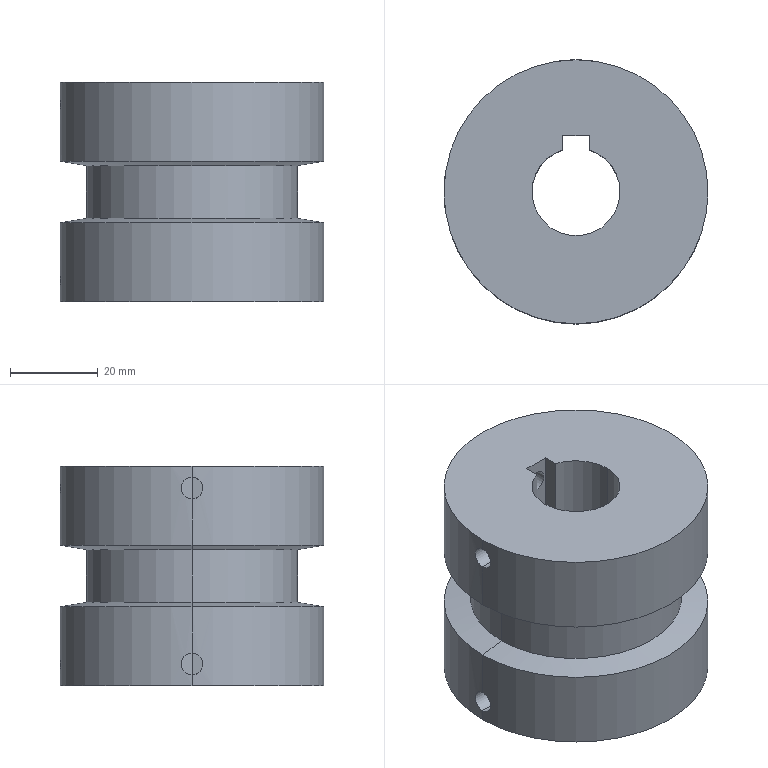Part | STEP file | ENE11-D60-N20-L50-X14-Y12-Z5 flat belt pulley Yihda 171 | 1 solid | 26 faces | box 60 x 60 x 50 mm | volume 110095 mm3 | cylinder 17 | plane 5 | cone 4 | commonest cylinder face diameters 4.917 x8 60 x4 20 x3 48 x2
STEP:
#1=CARTESIAN_POINT('',(-10.,0.,-50.));
#2=VERTEX_POINT('',#1);
#3=CARTESIAN_POINT('',(-3.,9.539,-50.));
#4=VERTEX_POINT('',#3);
#5=CARTESIAN_POINT('',(0.,0.,-50.));
#6=DIRECTION('',(0.,0.,-1.));
#7=DIRECTION('',(-1.,0.,0.));
#8=AXIS2_PLACEMENT_3D('',#5,#6,#7);
#9=CIRCLE('',#8,10.);
#10=EDGE_CURVE('',#2,#4,#9,.T.);
#11=ORIENTED_EDGE('',*,*,#10,.T.);
#12=CARTESIAN_POINT('',(-3.,9.539,0.));
#13=VERTEX_POINT('',#12);
#14=CARTESIAN_POINT('',(-3.,9.539,-50.));
#15=DIRECTION('',(0.,0.,1.));
#16=VECTOR('',#15,1000.);
#17=LINE('',#14,#16);
#18=EDGE_CURVE('',#4,#13,#17,.T.);
#19=ORIENTED_EDGE('',*,*,#18,.T.);
#20=CARTESIAN_POINT('',(-10.,0.,0.));
#21=VERTEX_POINT('',#20);
#22=CARTESIAN_POINT('',(0.,0.,0.));
#23=DIRECTION('',(0.,0.,-1.));
#24=DIRECTION('',(-1.,0.,0.));
#25=AXIS2_PLACEMENT_3D('',#22,#23,#24);
#26=CIRCLE('',#25,10.);
#27=EDGE_CURVE('',#21,#13,#26,.T.);
#28=ORIENTED_EDGE('',*,*,#27,.F.);
#29=CARTESIAN_POINT('',(-10.,0.,-2.542));
#30=VERTEX_POINT('',#29);
#31=CARTESIAN_POINT('',(-10.,0.,-2.542));
#32=DIRECTION('',(0.,0.,1.));
#33=VECTOR('',#32,1000.);
#34=LINE('',#31,#33);
#35=EDGE_CURVE('',#30,#21,#34,.T.);
#36=ORIENTED_EDGE('',*,*,#35,.F.);
#37=CARTESIAN_POINT('',(-10.,0.,-7.458));
#38=VERTEX_POINT('',#37);
#39=CARTESIAN_POINT('',(-10.,0.,-2.542));
#40=CARTESIAN_POINT('',(-10.,0.1631,-2.542));
#41=CARTESIAN_POINT('',(-9.996,0.3233,-2.558));
#42=CARTESIAN_POINT('',(-9.981,0.6386,-2.62));
#43=CARTESIAN_POINT('',(-9.969,0.795,-2.668));
#44=CARTESIAN_POINT('',(-9.941,1.092,-2.792));
#45=CARTESIAN_POINT('',(-9.925,1.233,-2.867));
#46=CARTESIAN_POINT('',(-9.888,1.5,-3.046));
#47=CARTESIAN_POINT('',(-9.868,1.626,-3.149));
#48=CARTESIAN_POINT('',(-9.808,1.965,-3.488));
#49=CARTESIAN_POINT('',(-9.768,2.148,-3.761));
#50=CARTESIAN_POINT('',(-9.725,2.332,-4.205));
#51=CARTESIAN_POINT('',(-9.713,2.379,-4.36));
#52=CARTESIAN_POINT('',(-9.697,2.443,-4.678));
#53=CARTESIAN_POINT('',(-9.693,2.458,-4.838));
#54=CARTESIAN_POINT('',(-9.693,2.459,-5.16));
#55=CARTESIAN_POINT('',(-9.697,2.442,-5.324));
#56=CARTESIAN_POINT('',(-9.713,2.379,-5.64));
#57=CARTESIAN_POINT('',(-9.724,2.333,-5.793));
#58=CARTESIAN_POINT('',(-9.768,2.147,-6.24));
#59=CARTESIAN_POINT('',(-9.808,1.966,-6.511));
#60=CARTESIAN_POINT('',(-9.868,1.624,-6.853));
#61=CARTESIAN_POINT('',(-9.888,1.501,-6.954));
#62=CARTESIAN_POINT('',(-9.924,1.235,-7.132));
#63=CARTESIAN_POINT('',(-9.941,1.091,-7.209));
#64=CARTESIAN_POINT('',(-9.97,0.7939,-7.332));
#65=CARTESIAN_POINT('',(-9.981,0.6406,-7.379));
#66=CARTESIAN_POINT('',(-9.996,0.3241,-7.442));
#67=CARTESIAN_POINT('',(-10.,0.1608,-7.459));
#68=CARTESIAN_POINT('',(-10.,0.,-7.458));
#69=B_SPLINE_CURVE_WITH_KNOTS('',3,(#39,#40,#41,#42,#43,#44,#45,#46,#47,#48,#49,#50,#51,#52,#53,#54,#55,#56,#57,#58,#59,#60,#61,#62,#63,#64,#65,#66,#67,#68),.UNSPECIFIED.,.F.,.F.,(4,2,2,2,2,2,2,2,2,2,2,2,2,2,4),(0.,0.0004823,0.0009645,0.001447,0.001929,0.002894,0.003376,0.003858,0.00434,0.004823,0.005787,0.006269,0.006752,0.007234,0.007716),.UNSPECIFIED.);
#70=EDGE_CURVE('',#30,#38,#69,.T.);
#71=ORIENTED_EDGE('',*,*,#70,.T.);
#72=CARTESIAN_POINT('',(-10.,-0.000000171,-7.458));
#73=VERTEX_POINT('',#72);
#74=CARTESIAN_POINT('',(-10.,0.,-7.458));
#75=DIRECTION('',(0.00006947,-1.,0.000000036));
#76=VECTOR('',#75,1000.);
#77=LINE('',#74,#76);
#78=EDGE_CURVE('',#38,#73,#77,.T.);
#79=ORIENTED_EDGE('',*,*,#78,.T.);
#80=CARTESIAN_POINT('',(-10.,0.,-42.542));
#81=VERTEX_POINT('',#80);
#82=CARTESIAN_POINT('',(-10.,0.,-42.542));
#83=DIRECTION('',(0.,0.,1.));
#84=VECTOR('',#83,1000.);
#85=LINE('',#82,#84);
#86=EDGE_CURVE('',#81,#73,#85,.T.);
#87=ORIENTED_EDGE('',*,*,#86,.F.);
#88=CARTESIAN_POINT('',(-10.,0.,-47.458));
#89=VERTEX_POINT('',#88);
#90=CARTESIAN_POINT('',(-10.,0.,-42.542));
#91=CARTESIAN_POINT('',(-10.,0.1631,-42.542));
#92=CARTESIAN_POINT('',(-9.996,0.3233,-42.558));
#93=CARTESIAN_POINT('',(-9.981,0.6386,-42.62));
#94=CARTESIAN_POINT('',(-9.969,0.795,-42.668));
#95=CARTESIAN_POINT('',(-9.941,1.092,-42.792));
#96=CARTESIAN_POINT('',(-9.925,1.233,-42.867));
#97=CARTESIAN_POINT('',(-9.888,1.5,-43.046));
#98=CARTESIAN_POINT('',(-9.868,1.626,-43.149));
#99=CARTESIAN_POINT('',(-9.808,1.965,-43.488));
#100=CARTESIAN_POINT('',(-9.768,2.148,-43.761));
#101=CARTESIAN_POINT('',(-9.725,2.332,-44.205));
#102=CARTESIAN_POINT('',(-9.713,2.379,-44.36));
#103=CARTESIAN_POINT('',(-9.697,2.443,-44.678));
#104=CARTESIAN_POINT('',(-9.693,2.458,-44.838));
#105=CARTESIAN_POINT('',(-9.693,2.459,-45.16));
#106=CARTESIAN_POINT('',(-9.697,2.442,-45.324));
#107=CARTESIAN_POINT('',(-9.713,2.379,-45.64));
#108=CARTESIAN_POINT('',(-9.724,2.333,-45.793));
#109=CARTESIAN_POINT('',(-9.768,2.147,-46.24));
#110=CARTESIAN_POINT('',(-9.808,1.966,-46.511));
#111=CARTESIAN_POINT('',(-9.868,1.624,-46.853));
#112=CARTESIAN_POINT('',(-9.888,1.501,-46.954));
#113=CARTESIAN_POINT('',(-9.924,1.235,-47.132));
#114=CARTESIAN_POINT('',(-9.941,1.091,-47.209));
#115=CARTESIAN_POINT('',(-9.97,0.7939,-47.332));
#116=CARTESIAN_POINT('',(-9.981,0.6406,-47.379));
#117=CARTESIAN_POINT('',(-9.996,0.324,-47.442));
#118=CARTESIAN_POINT('',(-10.,0.1611,-47.459));
#119=CARTESIAN_POINT('',(-10.,0.,-47.458));
#120=B_SPLINE_CURVE_WITH_KNOTS('',3,(#90,#91,#92,#93,#94,#95,#96,#97,#98,#99,#100,#101,#102,#103,#104,#105,#106,#107,#108,#109,#110,#111,#112,#113,#114,#115,#116,#117,#118,#119),.UNSPECIFIED.,.F.,.F.,(4,2,2,2,2,2,2,2,2,2,2,2,2,2,4),(0.,0.0004823,0.0009645,0.001447,0.001929,0.002894,0.003376,0.003858,0.00434,0.004823,0.005787,0.006269,0.006752,0.007234,0.007716),.UNSPECIFIED.);
#121=EDGE_CURVE('',#81,#89,#120,.T.);
#122=ORIENTED_EDGE('',*,*,#121,.T.);
#123=CARTESIAN_POINT('',(-10.,0.,-50.));
#124=DIRECTION('',(0.,0.,1.));
#125=VECTOR('',#124,1000.);
#126=LINE('',#123,#125);
#127=EDGE_CURVE('',#2,#89,#126,.T.);
#128=ORIENTED_EDGE('',*,*,#127,.F.);
#129=EDGE_LOOP('',(#11,#19,#28,#36,#71,#79,#87,#122,#128));
#130=FACE_OUTER_BOUND('',#129,.T.);
#131=CARTESIAN_POINT('',(0.,0.,-50.));
#132=DIRECTION('',(0.,0.,1.));
#133=DIRECTION('',(0.,-1.,0.));
#134=AXIS2_PLACEMENT_3D('',#131,#132,#133);
#135=CYLINDRICAL_SURFACE('',#134,10.);
#136=ADVANCED_FACE('',(#130),#135,.F.);
#137=ORIENTED_EDGE('',*,*,#70,.F.);
#138=CARTESIAN_POINT('',(-30.,0.,-2.541));
#139=VERTEX_POINT('',#138);
#140=CARTESIAN_POINT('',(-10.,0.,-2.542));
#141=DIRECTION('',(-1.,0.,0.));
#142=VECTOR('',#141,1000.);
#143=LINE('',#140,#142);
#144=EDGE_CURVE('',#30,#139,#143,.T.);
#145=ORIENTED_EDGE('',*,*,#144,.T.);
#146=CARTESIAN_POINT('',(-30.,0.,-7.458));
#147=VERTEX_POINT('',#146);
#148=CARTESIAN_POINT('',(-30.,0.,-7.458));
#149=CARTESIAN_POINT('',(-30.,0.1625,-7.458));
#150=CARTESIAN_POINT('',(-29.999,0.3222,-7.443));
#151=CARTESIAN_POINT('',(-29.994,0.6368,-7.38));
#152=CARTESIAN_POINT('',(-29.99,0.7928,-7.333));
#153=CARTESIAN_POINT('',(-29.981,1.091,-7.209));
#154=CARTESIAN_POINT('',(-29.975,1.232,-7.134));
#155=CARTESIAN_POINT('',(-29.963,1.499,-6.955));
#156=CARTESIAN_POINT('',(-29.956,1.625,-6.852));
#157=CARTESIAN_POINT('',(-29.943,1.852,-6.625));
#158=CARTESIAN_POINT('',(-29.936,1.954,-6.501));
#159=CARTESIAN_POINT('',(-29.924,2.133,-6.232));
#160=CARTESIAN_POINT('',(-29.919,2.21,-6.089));
#161=CARTESIAN_POINT('',(-29.909,2.333,-5.793));
#162=CARTESIAN_POINT('',(-29.905,2.38,-5.638));
#163=CARTESIAN_POINT('',(-29.9,2.443,-5.321));
#164=CARTESIAN_POINT('',(-29.899,2.458,-5.161));
#165=CARTESIAN_POINT('',(-29.899,2.459,-4.84));
#166=CARTESIAN_POINT('',(-29.9,2.443,-4.678));
#167=CARTESIAN_POINT('',(-29.905,2.38,-4.362));
#168=CARTESIAN_POINT('',(-29.909,2.333,-4.209));
#169=CARTESIAN_POINT('',(-29.919,2.21,-3.911));
#170=CARTESIAN_POINT('',(-29.924,2.133,-3.767));
#171=CARTESIAN_POINT('',(-29.936,1.955,-3.501));
#172=CARTESIAN_POINT('',(-29.943,1.853,-3.377));
#173=CARTESIAN_POINT('',(-29.956,1.624,-3.147));
#174=CARTESIAN_POINT('',(-29.963,1.5,-3.045));
#175=CARTESIAN_POINT('',(-29.975,1.233,-2.867));
#176=CARTESIAN_POINT('',(-29.981,1.09,-2.79));
#177=CARTESIAN_POINT('',(-29.99,0.792,-2.667));
#178=CARTESIAN_POINT('',(-29.994,0.6387,-2.62));
#179=CARTESIAN_POINT('',(-29.999,0.3234,-2.558));
#180=CARTESIAN_POINT('',(-30.,0.1606,-2.542));
#181=CARTESIAN_POINT('',(-30.,0.,-2.541));
#182=B_SPLINE_CURVE_WITH_KNOTS('',3,(#148,#149,#150,#151,#152,#153,#154,#155,#156,#157,#158,#159,#160,#161,#162,#163,#164,#165,#166,#167,#168,#169,#170,#171,#172,#173,#174,#175,#176,#177,#178,#179,#180,#181),.UNSPECIFIED.,.F.,.F.,(4,2,2,2,2,2,2,2,2,2,2,2,2,2,2,2,4),(0.,0.0004806,0.0009612,0.001442,0.001922,0.002403,0.002884,0.003364,0.003845,0.004325,0.004806,0.005287,0.005767,0.006248,0.006728,0.007209,0.00769),.UNSPECIFIED.);
#183=EDGE_CURVE('',#147,#139,#182,.T.);
#184=ORIENTED_EDGE('',*,*,#183,.F.);
#185=CARTESIAN_POINT('',(-10.,0.,-7.458));
#186=DIRECTION('',(-1.,0.,0.));
#187=VECTOR('',#186,1000.);
#188=LINE('',#185,#187);
#189=EDGE_CURVE('',#38,#147,#188,.T.);
#190=ORIENTED_EDGE('',*,*,#189,.F.);
#191=EDGE_LOOP('',(#137,#145,#184,#190));
#192=FACE_OUTER_BOUND('',#191,.T.);
#193=CARTESIAN_POINT('',(0.,0.,-5.));
#194=DIRECTION('',(-1.,0.,0.));
#195=DIRECTION('',(0.,-1.,0.));
#196=AXIS2_PLACEMENT_3D('',#193,#194,#195);
#197=CYLINDRICAL_SURFACE('',#196,2.459);
#198=ADVANCED_FACE('',(#192),#197,.F.);
#199=CARTESIAN_POINT('',(-30.,0.,-2.541));
#200=CARTESIAN_POINT('',(-30.,-0.1606,-2.541));
#201=CARTESIAN_POINT('',(-29.999,-0.3201,-2.557));
#202=CARTESIAN_POINT('',(-29.994,-0.6369,-2.62));
#203=CARTESIAN_POINT('',(-29.99,-0.7923,-2.667));
#204=CARTESIAN_POINT('',(-29.976,-1.236,-2.851));
#205=CARTESIAN_POINT('',(-29.963,-1.51,-3.034));
#206=CARTESIAN_POINT('',(-29.943,-1.851,-3.374));
#207=CARTESIAN_POINT('',(-29.936,-1.954,-3.5));
#208=CARTESIAN_POINT('',(-29.924,-2.133,-3.767));
#209=CARTESIAN_POINT('',(-29.919,-2.209,-3.908));
#210=CARTESIAN_POINT('',(-29.909,-2.332,-4.206));
#211=CARTESIAN_POINT('',(-29.905,-2.38,-4.362));
#212=CARTESIAN_POINT('',(-29.9,-2.442,-4.676));
#213=CARTESIAN_POINT('',(-29.899,-2.458,-4.836));
#214=CARTESIAN_POINT('',(-29.899,-2.459,-5.16));
#215=CARTESIAN_POINT('',(-29.9,-2.443,-5.32));
#216=CARTESIAN_POINT('',(-29.905,-2.38,-5.635));
#217=CARTESIAN_POINT('',(-29.909,-2.333,-5.791));
#218=CARTESIAN_POINT('',(-29.919,-2.21,-6.089));
#219=CARTESIAN_POINT('',(-29.924,-2.135,-6.23));
#220=CARTESIAN_POINT('',(-29.936,-1.957,-6.497));
#221=CARTESIAN_POINT('',(-29.943,-1.853,-6.624));
#222=CARTESIAN_POINT('',(-29.956,-1.626,-6.851));
#223=CARTESIAN_POINT('',(-29.963,-1.503,-6.953));
#224=CARTESIAN_POINT('',(-29.975,-1.234,-7.132));
#225=CARTESIAN_POINT('',(-29.981,-1.091,-7.209));
#226=CARTESIAN_POINT('',(-29.994,-0.6476,-7.393));
#227=CARTESIAN_POINT('',(-30.,-0.3249,-7.458));
#228=CARTESIAN_POINT('',(-30.,0.,-7.458));
#229=B_SPLINE_CURVE_WITH_KNOTS('',3,(#199,#200,#201,#202,#203,#204,#205,#206,#207,#208,#209,#210,#211,#212,#213,#214,#215,#216,#217,#218,#219,#220,#221,#222,#223,#224,#225,#226,#227,#228),.UNSPECIFIED.,.F.,.F.,(4,2,2,2,2,2,2,2,2,2,2,2,2,2,4),(0.00769,0.00817,0.008651,0.009612,0.01009,0.01057,0.01105,0.01153,0.01201,0.01249,0.01297,0.01346,0.01394,0.01442,0.01538),.UNSPECIFIED.);
#230=EDGE_CURVE('',#139,#147,#229,.T.);
#231=ORIENTED_EDGE('',*,*,#230,.F.);
#232=ORIENTED_EDGE('',*,*,#144,.F.);
#233=CARTESIAN_POINT('',(-10.,-0.000000171,-7.458));
#234=CARTESIAN_POINT('',(-10.,-0.3216,-7.458));
#235=CARTESIAN_POINT('',(-9.984,-0.6459,-7.394));
#236=CARTESIAN_POINT('',(-9.941,-1.091,-7.209));
#237=CARTESIAN_POINT('',(-9.924,-1.234,-7.132));
#238=CARTESIAN_POINT('',(-9.888,-1.501,-6.954));
#239=CARTESIAN_POINT('',(-9.868,-1.624,-6.852));
#240=CARTESIAN_POINT('',(-9.828,-1.851,-6.626));
#241=CARTESIAN_POINT('',(-9.808,-1.954,-6.5));
#242=CARTESIAN_POINT('',(-9.77,-2.132,-6.234));
#243=CARTESIAN_POINT('',(-9.753,-2.208,-6.093));
#244=CARTESIAN_POINT('',(-9.71,-2.394,-5.645));
#245=CARTESIAN_POINT('',(-9.693,-2.458,-5.325));
#246=CARTESIAN_POINT('',(-9.693,-2.459,-4.839));
#247=CARTESIAN_POINT('',(-9.697,-2.443,-4.679));
#248=CARTESIAN_POINT('',(-9.713,-2.38,-4.363));
#249=CARTESIAN_POINT('',(-9.724,-2.332,-4.206));
#250=CARTESIAN_POINT('',(-9.753,-2.209,-3.909));
#251=CARTESIAN_POINT('',(-9.77,-2.134,-3.768));
#252=CARTESIAN_POINT('',(-9.807,-1.955,-3.5));
#253=CARTESIAN_POINT('',(-9.828,-1.852,-3.376));
#254=CARTESIAN_POINT('',(-9.887,-1.514,-3.037));
#255=CARTESIAN_POINT('',(-9.927,-1.241,-2.854));
#256=CARTESIAN_POINT('',(-9.969,-0.7971,-2.669));
#257=CARTESIAN_POINT('',(-9.981,-0.6407,-2.621));
#258=CARTESIAN_POINT('',(-9.996,-0.3238,-2.558));
#259=CARTESIAN_POINT('',(-10.,-0.1631,-2.542));
#260=CARTESIAN_POINT('',(-10.,0.,-2.542));
#261=B_SPLINE_CURVE_WITH_KNOTS('',3,(#233,#234,#235,#236,#237,#238,#239,#240,#241,#242,#243,#244,#245,#246,#247,#248,#249,#250,#251,#252,#253,#254,#255,#256,#257,#258,#259,#260),.UNSPECIFIED.,.F.,.F.,(4,2,2,2,2,2,2,2,2,2,2,2,2,4),(0.007716,0.00868,0.009162,0.009645,0.01013,0.01061,0.01157,0.01206,0.01254,0.01302,0.0135,0.01447,0.01495,0.01543),.UNSPECIFIED.);
#262=EDGE_CURVE('',#73,#30,#261,.T.);
#263=ORIENTED_EDGE('',*,*,#262,.F.);
#264=ORIENTED_EDGE('',*,*,#78,.F.);
#265=ORIENTED_EDGE('',*,*,#189,.T.);
#266=EDGE_LOOP('',(#231,#232,#263,#264,#265));
#267=FACE_OUTER_BOUND('',#266,.T.);
#268=CARTESIAN_POINT('',(0.,0.,-5.));
#269=DIRECTION('',(-1.,0.,0.));
#270=DIRECTION('',(0.,1.,0.));
#271=AXIS2_PLACEMENT_3D('',#268,#269,#270);
#272=CYLINDRICAL_SURFACE('',#271,2.459);
#273=ADVANCED_FACE('',(#267),#272,.F.);
#274=CARTESIAN_POINT('',(3.,9.539,0.));
#275=VERTEX_POINT('',#274);
#276=CARTESIAN_POINT('',(10.,0.,0.));
#277=VERTEX_POINT('',#276);
#278=CARTESIAN_POINT('',(0.,0.,0.));
#279=DIRECTION('',(0.,0.,-1.));
#280=DIRECTION('',(-1.,0.,0.));
#281=AXIS2_PLACEMENT_3D('',#278,#279,#280);
#282=CIRCLE('',#281,10.);
#283=EDGE_CURVE('',#275,#277,#282,.T.);
#284=ORIENTED_EDGE('',*,*,#283,.F.);
#285=CARTESIAN_POINT('',(3.,9.539,-50.));
#286=VERTEX_POINT('',#285);
#287=CARTESIAN_POINT('',(3.,9.539,-50.));
#288=DIRECTION('',(0.,0.,-1.));
#289=VECTOR('',#288,1000.);
#290=LINE('',#287,#289);
#291=EDGE_CURVE('',#275,#286,#290,.T.);
#292=ORIENTED_EDGE('',*,*,#291,.T.);
#293=CARTESIAN_POINT('',(10.,0.,-50.));
#294=VERTEX_POINT('',#293);
#295=CARTESIAN_POINT('',(0.,0.,-50.));
#296=DIRECTION('',(0.,0.,-1.));
#297=DIRECTION('',(-1.,0.,0.));
#298=AXIS2_PLACEMENT_3D('',#295,#296,#297);
#299=CIRCLE('',#298,10.);
#300=EDGE_CURVE('',#286,#294,#299,.T.);
#301=ORIENTED_EDGE('',*,*,#300,.T.);
#302=CARTESIAN_POINT('',(10.,0.,-50.));
#303=DIRECTION('',(0.,0.,1.));
#304=VECTOR('',#303,1000.);
#305=LINE('',#302,#304);
#306=EDGE_CURVE('',#294,#277,#305,.T.);
#307=ORIENTED_EDGE('',*,*,#306,.T.);
#308=EDGE_LOOP('',(#284,#292,#301,#307));
#309=FACE_OUTER_BOUND('',#308,.T.);
#310=CARTESIAN_POINT('',(0.,0.,-50.));
#311=DIRECTION('',(0.,0.,1.));
#312=DIRECTION('',(0.,-1.,0.));
#313=AXIS2_PLACEMENT_3D('',#310,#311,#312);
#314=CYLINDRICAL_SURFACE('',#313,10.);
#315=ADVANCED_FACE('',(#309),#314,.F.);
#316=CARTESIAN_POINT('',(0.,12.8,-7.458));
#317=VERTEX_POINT('',#316);
#318=CARTESIAN_POINT('',(0.,30.,-7.458));
#319=VERTEX_POINT('',#318);
#320=CARTESIAN_POINT('',(0.,10.,-7.458));
#321=DIRECTION('',(0.,1.,0.));
#322=VECTOR('',#321,1000.);
#323=LINE('',#320,#322);
#324=EDGE_CURVE('',#317,#319,#323,.T.);
#325=ORIENTED_EDGE('',*,*,#324,.F.);
#326=CARTESIAN_POINT('',(0.,12.8,-2.542));
#327=VERTEX_POINT('',#326);
#328=CARTESIAN_POINT('',(0.,12.8,-5.));
#329=DIRECTION('',(0.,-1.,0.));
#330=DIRECTION('',(0.,0.,1.));
#331=AXIS2_PLACEMENT_3D('',#328,#329,#330);
#332=CIRCLE('',#331,2.459);
#333=EDGE_CURVE('',#317,#327,#332,.T.);
#334=ORIENTED_EDGE('',*,*,#333,.T.);
#335=CARTESIAN_POINT('',(0.,30.,-2.542));
#336=VERTEX_POINT('',#335);
#337=CARTESIAN_POINT('',(0.,10.,-2.542));
#338=DIRECTION('',(0.,1.,0.));
#339=VECTOR('',#338,1000.);
#340=LINE('',#337,#339);
#341=EDGE_CURVE('',#327,#336,#340,.T.);
#342=ORIENTED_EDGE('',*,*,#341,.T.);
#343=CARTESIAN_POINT('',(0.,30.,-7.458));
#344=CARTESIAN_POINT('',(0.1625,30.,-7.459));
#345=CARTESIAN_POINT('',(0.3222,29.999,-7.443));
#346=CARTESIAN_POINT('',(0.6368,29.994,-7.38));
#347=CARTESIAN_POINT('',(0.7928,29.99,-7.333));
#348=CARTESIAN_POINT('',(1.091,29.981,-7.209));
#349=CARTESIAN_POINT('',(1.232,29.975,-7.134));
#350=CARTESIAN_POINT('',(1.499,29.963,-6.955));
#351=CARTESIAN_POINT('',(1.625,29.956,-6.852));
#352=CARTESIAN_POINT('',(1.852,29.943,-6.625));
#353=CARTESIAN_POINT('',(1.954,29.936,-6.501));
#354=CARTESIAN_POINT('',(2.133,29.924,-6.232));
#355=CARTESIAN_POINT('',(2.21,29.919,-6.089));
#356=CARTESIAN_POINT('',(2.333,29.909,-5.793));
#357=CARTESIAN_POINT('',(2.38,29.905,-5.638));
#358=CARTESIAN_POINT('',(2.443,29.9,-5.321));
#359=CARTESIAN_POINT('',(2.458,29.899,-5.161));
#360=CARTESIAN_POINT('',(2.459,29.899,-4.84));
#361=CARTESIAN_POINT('',(2.443,29.9,-4.678));
#362=CARTESIAN_POINT('',(2.38,29.905,-4.362));
#363=CARTESIAN_POINT('',(2.333,29.909,-4.209));
#364=CARTESIAN_POINT('',(2.21,29.919,-3.911));
#365=CARTESIAN_POINT('',(2.133,29.924,-3.767));
#366=CARTESIAN_POINT('',(1.955,29.936,-3.501));
#367=CARTESIAN_POINT('',(1.853,29.943,-3.377));
#368=CARTESIAN_POINT('',(1.624,29.956,-3.147));
#369=CARTESIAN_POINT('',(1.5,29.963,-3.045));
#370=CARTESIAN_POINT('',(1.233,29.975,-2.867));
#371=CARTESIAN_POINT('',(1.09,29.981,-2.79));
#372=CARTESIAN_POINT('',(0.792,29.99,-2.667));
#373=CARTESIAN_POINT('',(0.6387,29.994,-2.62));
#374=CARTESIAN_POINT('',(0.3234,29.999,-2.558));
#375=CARTESIAN_POINT('',(0.1606,30.,-2.542));
#376=CARTESIAN_POINT('',(0.,30.,-2.542));
#377=B_SPLINE_CURVE_WITH_KNOTS('',3,(#343,#344,#345,#346,#347,#348,#349,#350,#351,#352,#353,#354,#355,#356,#357,#358,#359,#360,#361,#362,#363,#364,#365,#366,#367,#368,#369,#370,#371,#372,#373,#374,#375,#376),.UNSPECIFIED.,.F.,.F.,(4,2,2,2,2,2,2,2,2,2,2,2,2,2,2,2,4),(0.,0.0004806,0.0009612,0.001442,0.001922,0.002403,0.002884,0.003364,0.003845,0.004325,0.004806,0.005287,0.005767,0.006248,0.006728,0.007209,0.00769),.UNSPECIFIED.);
#378=EDGE_CURVE('',#319,#336,#377,.T.);
#379=ORIENTED_EDGE('',*,*,#378,.F.);
#380=EDGE_LOOP('',(#325,#334,#342,#379));
#381=FACE_OUTER_BOUND('',#380,.T.);
#382=CARTESIAN_POINT('',(0.,0.,-5.));
#383=DIRECTION('',(0.,1.,0.));
#384=DIRECTION('',(-1.,0.,0.));
#385=AXIS2_PLACEMENT_3D('',#382,#383,#384);
#386=CYLINDRICAL_SURFACE('',#385,2.459);
#387=ADVANCED_FACE('',(#381),#386,.F.);
#388=ORIENTED_EDGE('',*,*,#341,.F.);
#389=CARTESIAN_POINT('',(0.,12.8,-5.));
#390=DIRECTION('',(0.,-1.,0.));
#391=DIRECTION('',(0.,0.,1.));
#392=AXIS2_PLACEMENT_3D('',#389,#390,#391);
#393=CIRCLE('',#392,2.459);
#394=EDGE_CURVE('',#327,#317,#393,.T.);
#395=ORIENTED_EDGE('',*,*,#394,.T.);
#396=ORIENTED_EDGE('',*,*,#324,.T.);
#397=CARTESIAN_POINT('',(0.,30.,-2.542));
#398=CARTESIAN_POINT('',(-0.1606,30.,-2.541));
#399=CARTESIAN_POINT('',(-0.3201,29.999,-2.557));
#400=CARTESIAN_POINT('',(-0.6369,29.994,-2.62));
#401=CARTESIAN_POINT('',(-0.7923,29.99,-2.667));
#402=CARTESIAN_POINT('',(-1.236,29.976,-2.851));
#403=CARTESIAN_POINT('',(-1.51,29.963,-3.034));
#404=CARTESIAN_POINT('',(-1.851,29.943,-3.374));
#405=CARTESIAN_POINT('',(-1.954,29.936,-3.5));
#406=CARTESIAN_POINT('',(-2.133,29.924,-3.767));
#407=CARTESIAN_POINT('',(-2.209,29.919,-3.908));
#408=CARTESIAN_POINT('',(-2.332,29.909,-4.206));
#409=CARTESIAN_POINT('',(-2.38,29.905,-4.362));
#410=CARTESIAN_POINT('',(-2.442,29.9,-4.676));
#411=CARTESIAN_POINT('',(-2.458,29.899,-4.836));
#412=CARTESIAN_POINT('',(-2.459,29.899,-5.16));
#413=CARTESIAN_POINT('',(-2.443,29.9,-5.32));
#414=CARTESIAN_POINT('',(-2.38,29.905,-5.635));
#415=CARTESIAN_POINT('',(-2.333,29.909,-5.791));
#416=CARTESIAN_POINT('',(-2.21,29.919,-6.089));
#417=CARTESIAN_POINT('',(-2.135,29.924,-6.23));
#418=CARTESIAN_POINT('',(-1.957,29.936,-6.497));
#419=CARTESIAN_POINT('',(-1.853,29.943,-6.624));
#420=CARTESIAN_POINT('',(-1.626,29.956,-6.851));
#421=CARTESIAN_POINT('',(-1.503,29.963,-6.953));
#422=CARTESIAN_POINT('',(-1.234,29.975,-7.132));
#423=CARTESIAN_POINT('',(-1.091,29.981,-7.209));
#424=CARTESIAN_POINT('',(-0.6476,29.994,-7.393));
#425=CARTESIAN_POINT('',(-0.3249,30.,-7.459));
#426=CARTESIAN_POINT('',(0.,30.,-7.458));
#427=B_SPLINE_CURVE_WITH_KNOTS('',3,(#397,#398,#399,#400,#401,#402,#403,#404,#405,#406,#407,#408,#409,#410,#411,#412,#413,#414,#415,#416,#417,#418,#419,#420,#421,#422,#423,#424,#425,#426),.UNSPECIFIED.,.F.,.F.,(4,2,2,2,2,2,2,2,2,2,2,2,2,2,4),(0.00769,0.00817,0.008651,0.009612,0.01009,0.01057,0.01105,0.01153,0.01201,0.01249,0.01297,0.01346,0.01394,0.01442,0.01538),.UNSPECIFIED.);
#428=EDGE_CURVE('',#336,#319,#427,.T.);
#429=ORIENTED_EDGE('',*,*,#428,.F.);
#430=EDGE_LOOP('',(#388,#395,#396,#429));
#431=FACE_OUTER_BOUND('',#430,.T.);
#432=CARTESIAN_POINT('',(0.,0.,-5.));
#433=DIRECTION('',(0.,1.,0.));
#434=DIRECTION('',(1.,0.,0.));
#435=AXIS2_PLACEMENT_3D('',#432,#433,#434);
#436=CYLINDRICAL_SURFACE('',#435,2.459);
#437=ADVANCED_FACE('',(#431),#436,.F.);
#438=CARTESIAN_POINT('',(-30.,0.,-18.));
#439=VERTEX_POINT('',#438);
#440=CARTESIAN_POINT('',(30.,0.,-18.));
#441=VERTEX_POINT('',#440);
#442=CARTESIAN_POINT('',(0.,0.,-18.));
#443=DIRECTION('',(0.,0.,-1.));
#444=DIRECTION('',(-1.,0.,0.));
#445=AXIS2_PLACEMENT_3D('',#442,#443,#444);
#446=CIRCLE('',#445,30.);
#447=EDGE_CURVE('',#439,#441,#446,.T.);
#448=ORIENTED_EDGE('',*,*,#447,.F.);
#449=CARTESIAN_POINT('',(-30.,0.,-18.));
#450=DIRECTION('',(0.,0.,1.));
#451=VECTOR('',#450,1000.);
#452=LINE('',#449,#451);
#453=EDGE_CURVE('',#439,#147,#452,.T.);
#454=ORIENTED_EDGE('',*,*,#453,.T.);
#455=ORIENTED_EDGE('',*,*,#183,.T.);
#456=CARTESIAN_POINT('',(-30.,0.,0.));
#457=VERTEX_POINT('',#456);
#458=CARTESIAN_POINT('',(-30.,0.,-2.541));
#459=DIRECTION('',(0.,0.,1.));
#460=VECTOR('',#459,1000.);
#461=LINE('',#458,#460);
#462=EDGE_CURVE('',#139,#457,#461,.T.);
#463=ORIENTED_EDGE('',*,*,#462,.T.);
#464=CARTESIAN_POINT('',(30.,0.,0.));
#465=VERTEX_POINT('',#464);
#466=CARTESIAN_POINT('',(0.,0.,0.));
#467=DIRECTION('',(0.,0.,-1.));
#468=DIRECTION('',(-1.,0.,0.));
#469=AXIS2_PLACEMENT_3D('',#466,#467,#468);
#470=CIRCLE('',#469,30.);
#471=EDGE_CURVE('',#457,#465,#470,.T.);
#472=ORIENTED_EDGE('',*,*,#471,.T.);
#473=CARTESIAN_POINT('',(30.,0.,-18.));
#474=DIRECTION('',(0.,0.,1.));
#475=VECTOR('',#474,1000.);
#476=LINE('',#473,#475);
#477=EDGE_CURVE('',#441,#465,#476,.T.);
#478=ORIENTED_EDGE('',*,*,#477,.F.);
#479=EDGE_LOOP('',(#448,#454,#455,#463,#472,#478));
#480=FACE_OUTER_BOUND('',#479,.T.);
#481=ORIENTED_EDGE('',*,*,#378,.T.);
#482=ORIENTED_EDGE('',*,*,#428,.T.);
#483=EDGE_LOOP('',(#481,#482));
#484=FACE_BOUND('',#483,.T.);
#485=CARTESIAN_POINT('',(0.,0.,-50.));
#486=DIRECTION('',(0.,0.,1.));
#487=DIRECTION('',(0.,-1.,0.));
#488=AXIS2_PLACEMENT_3D('',#485,#486,#487);
#489=CYLINDRICAL_SURFACE('',#488,30.);
#490=ADVANCED_FACE('',(#480,#484),#489,.T.);
#491=CARTESIAN_POINT('',(0.,0.,0.));
#492=DIRECTION('',(0.,0.,-1.));
#493=DIRECTION('',(-1.,0.,0.));
#494=AXIS2_PLACEMENT_3D('',#491,#492,#493);
#495=CIRCLE('',#494,30.);
#496=EDGE_CURVE('',#465,#457,#495,.T.);
#497=ORIENTED_EDGE('',*,*,#496,.T.);
#498=ORIENTED_EDGE('',*,*,#462,.F.);
#499=ORIENTED_EDGE('',*,*,#230,.T.);
#500=ORIENTED_EDGE('',*,*,#453,.F.);
#501=CARTESIAN_POINT('',(0.,0.,-18.));
#502=DIRECTION('',(0.,0.,-1.));
#503=DIRECTION('',(-1.,0.,0.));
#504=AXIS2_PLACEMENT_3D('',#501,#502,#503);
#505=CIRCLE('',#504,30.);
#506=EDGE_CURVE('',#441,#439,#505,.T.);
#507=ORIENTED_EDGE('',*,*,#506,.F.);
#508=ORIENTED_EDGE('',*,*,#477,.T.);
#509=EDGE_LOOP('',(#497,#498,#499,#500,#507,#508));
#510=FACE_OUTER_BOUND('',#509,.T.);
#511=CARTESIAN_POINT('',(0.,0.,-50.));
#512=DIRECTION('',(0.,0.,1.));
#513=DIRECTION('',(0.,1.,0.));
#514=AXIS2_PLACEMENT_3D('',#511,#512,#513);
#515=CYLINDRICAL_SURFACE('',#514,30.);
#516=ADVANCED_FACE('',(#510),#515,.T.);
#517=ORIENTED_EDGE('',*,*,#506,.T.);
#518=CARTESIAN_POINT('',(-24.,0.,-19.));
#519=VERTEX_POINT('',#518);
#520=CARTESIAN_POINT('',(-24.,0.,-19.));
#521=DIRECTION('',(-0.9864,0.,0.1644));
#522=VECTOR('',#521,1000.);
#523=LINE('',#520,#522);
#524=EDGE_CURVE('',#519,#439,#523,.T.);
#525=ORIENTED_EDGE('',*,*,#524,.F.);
#526=CARTESIAN_POINT('',(24.,0.,-19.));
#527=VERTEX_POINT('',#526);
#528=CARTESIAN_POINT('',(0.,0.,-19.));
#529=DIRECTION('',(0.,0.,-1.));
#530=DIRECTION('',(-1.,0.,0.));
#531=AXIS2_PLACEMENT_3D('',#528,#529,#530);
#532=CIRCLE('',#531,24.);
#533=EDGE_CURVE('',#527,#519,#532,.T.);
#534=ORIENTED_EDGE('',*,*,#533,.F.);
#535=CARTESIAN_POINT('',(24.,0.,-19.));
#536=DIRECTION('',(0.9864,0.,0.1644));
#537=VECTOR('',#536,1000.);
#538=LINE('',#535,#537);
#539=EDGE_CURVE('',#527,#441,#538,.T.);
#540=ORIENTED_EDGE('',*,*,#539,.T.);
#541=EDGE_LOOP('',(#517,#525,#534,#540));
#542=FACE_OUTER_BOUND('',#541,.T.);
#543=CARTESIAN_POINT('',(0.,0.,-18.));
#544=DIRECTION('',(0.,0.,1.));
#545=DIRECTION('',(0.,1.,0.));
#546=AXIS2_PLACEMENT_3D('',#543,#544,#545);
#547=CONICAL_SURFACE('',#546,30.,1.406);
#548=ADVANCED_FACE('',(#542),#547,.T.);
#549=CARTESIAN_POINT('',(0.,0.,-19.));
#550=DIRECTION('',(0.,0.,-1.));
#551=DIRECTION('',(-1.,0.,0.));
#552=AXIS2_PLACEMENT_3D('',#549,#550,#551);
#553=CIRCLE('',#552,24.);
#554=EDGE_CURVE('',#519,#527,#553,.T.);
#555=ORIENTED_EDGE('',*,*,#554,.F.);
#556=ORIENTED_EDGE('',*,*,#524,.T.);
#557=ORIENTED_EDGE('',*,*,#447,.T.);
#558=ORIENTED_EDGE('',*,*,#539,.F.);
#559=EDGE_LOOP('',(#555,#556,#557,#558));
#560=FACE_OUTER_BOUND('',#559,.T.);
#561=CARTESIAN_POINT('',(0.,0.,-18.));
#562=DIRECTION('',(0.,0.,1.));
#563=DIRECTION('',(0.,-1.,0.));
#564=AXIS2_PLACEMENT_3D('',#561,#562,#563);
#565=CONICAL_SURFACE('',#564,30.,1.406);
#566=ADVANCED_FACE('',(#560),#565,.T.);
#567=CARTESIAN_POINT('',(-24.,0.,-31.));
#568=VERTEX_POINT('',#567);
#569=CARTESIAN_POINT('',(24.,0.,-31.));
#570=VERTEX_POINT('',#569);
#571=CARTESIAN_POINT('',(0.,0.,-31.));
#572=DIRECTION('',(0.,0.,-1.));
#573=DIRECTION('',(-1.,0.,0.));
#574=AXIS2_PLACEMENT_3D('',#571,#572,#573);
#575=CIRCLE('',#574,24.);
#576=EDGE_CURVE('',#568,#570,#575,.T.);
#577=ORIENTED_EDGE('',*,*,#576,.F.);
#578=CARTESIAN_POINT('',(-24.,0.,-31.));
#579=DIRECTION('',(0.,0.,1.));
#580=VECTOR('',#579,1000.);
#581=LINE('',#578,#580);
#582=EDGE_CURVE('',#568,#519,#581,.T.);
#583=ORIENTED_EDGE('',*,*,#582,.T.);
#584=ORIENTED_EDGE('',*,*,#554,.T.);
#585=CARTESIAN_POINT('',(24.,0.,-31.));
#586=DIRECTION('',(0.,0.,1.));
#587=VECTOR('',#586,1000.);
#588=LINE('',#585,#587);
#589=EDGE_CURVE('',#570,#527,#588,.T.);
#590=ORIENTED_EDGE('',*,*,#589,.F.);
#591=EDGE_LOOP('',(#577,#583,#584,#590));
#592=FACE_OUTER_BOUND('',#591,.T.);
#593=CARTESIAN_POINT('',(0.,0.,-50.));
#594=DIRECTION('',(0.,0.,1.));
#595=DIRECTION('',(0.,-1.,0.));
#596=AXIS2_PLACEMENT_3D('',#593,#594,#595);
#597=CYLINDRICAL_SURFACE('',#596,24.);
#598=ADVANCED_FACE('',(#592),#597,.T.);
#599=ORIENTED_EDGE('',*,*,#533,.T.);
#600=ORIENTED_EDGE('',*,*,#582,.F.);
#601=CARTESIAN_POINT('',(0.,0.,-31.));
#602=DIRECTION('',(0.,0.,-1.));
#603=DIRECTION('',(-1.,0.,0.));
#604=AXIS2_PLACEMENT_3D('',#601,#602,#603);
#605=CIRCLE('',#604,24.);
#606=EDGE_CURVE('',#570,#568,#605,.T.);
#607=ORIENTED_EDGE('',*,*,#606,.F.);
#608=ORIENTED_EDGE('',*,*,#589,.T.);
#609=EDGE_LOOP('',(#599,#600,#607,#608));
#610=FACE_OUTER_BOUND('',#609,.T.);
#611=CARTESIAN_POINT('',(0.,0.,-50.));
#612=DIRECTION('',(0.,0.,1.));
#613=DIRECTION('',(0.,1.,0.));
#614=AXIS2_PLACEMENT_3D('',#611,#612,#613);
#615=CYLINDRICAL_SURFACE('',#614,24.);
#616=ADVANCED_FACE('',(#610),#615,.T.);
#617=ORIENTED_EDGE('',*,*,#606,.T.);
#618=CARTESIAN_POINT('',(-30.,0.,-32.));
#619=VERTEX_POINT('',#618);
#620=CARTESIAN_POINT('',(-24.,0.,-31.));
#621=DIRECTION('',(-0.9864,0.,-0.1644));
#622=VECTOR('',#621,1000.);
#623=LINE('',#620,#622);
#624=EDGE_CURVE('',#568,#619,#623,.T.);
#625=ORIENTED_EDGE('',*,*,#624,.T.);
#626=CARTESIAN_POINT('',(30.,0.,-32.));
#627=VERTEX_POINT('',#626);
#628=CARTESIAN_POINT('',(0.,0.,-32.));
#629=DIRECTION('',(0.,0.,-1.));
#630=DIRECTION('',(-1.,0.,0.));
#631=AXIS2_PLACEMENT_3D('',#628,#629,#630);
#632=CIRCLE('',#631,30.);
#633=EDGE_CURVE('',#627,#619,#632,.T.);
#634=ORIENTED_EDGE('',*,*,#633,.F.);
#635=CARTESIAN_POINT('',(24.,0.,-31.));
#636=DIRECTION('',(0.9864,0.,-0.1644));
#637=VECTOR('',#636,1000.);
#638=LINE('',#635,#637);
#639=EDGE_CURVE('',#570,#627,#638,.T.);
#640=ORIENTED_EDGE('',*,*,#639,.F.);
#641=EDGE_LOOP('',(#617,#625,#634,#640));
#642=FACE_OUTER_BOUND('',#641,.T.);
#643=CARTESIAN_POINT('',(0.,0.,-31.));
#644=DIRECTION('',(0.,0.,-1.));
#645=DIRECTION('',(0.,1.,0.));
#646=AXIS2_PLACEMENT_3D('',#643,#644,#645);
#647=CONICAL_SURFACE('',#646,24.,1.406);
#648=ADVANCED_FACE('',(#642),#647,.T.);
#649=CARTESIAN_POINT('',(0.,0.,-32.));
#650=DIRECTION('',(0.,0.,-1.));
#651=DIRECTION('',(-1.,0.,0.));
#652=AXIS2_PLACEMENT_3D('',#649,#650,#651);
#653=CIRCLE('',#652,30.);
#654=EDGE_CURVE('',#619,#627,#653,.T.);
#655=ORIENTED_EDGE('',*,*,#654,.F.);
#656=ORIENTED_EDGE('',*,*,#624,.F.);
#657=ORIENTED_EDGE('',*,*,#576,.T.);
#658=ORIENTED_EDGE('',*,*,#639,.T.);
#659=EDGE_LOOP('',(#655,#656,#657,#658));
#660=FACE_OUTER_BOUND('',#659,.T.);
#661=CARTESIAN_POINT('',(0.,0.,-31.));
#662=DIRECTION('',(0.,0.,-1.));
#663=DIRECTION('',(0.,-1.,0.));
#664=AXIS2_PLACEMENT_3D('',#661,#662,#663);
#665=CONICAL_SURFACE('',#664,24.,1.406);
#666=ADVANCED_FACE('',(#660),#665,.T.);
#667=CARTESIAN_POINT('',(-30.,0.,-50.));
#668=VERTEX_POINT('',#667);
#669=CARTESIAN_POINT('',(30.,0.,-50.));
#670=VERTEX_POINT('',#669);
#671=CARTESIAN_POINT('',(0.,0.,-50.));
#672=DIRECTION('',(0.,0.,-1.));
#673=DIRECTION('',(-1.,0.,0.));
#674=AXIS2_PLACEMENT_3D('',#671,#672,#673);
#675=CIRCLE('',#674,30.);
#676=EDGE_CURVE('',#668,#670,#675,.T.);
#677=ORIENTED_EDGE('',*,*,#676,.F.);
#678=CARTESIAN_POINT('',(-30.,0.,-47.459));
#679=VERTEX_POINT('',#678);
#680=CARTESIAN_POINT('',(-30.,0.,-50.));
#681=DIRECTION('',(0.,0.,1.));
#682=VECTOR('',#681,1000.);
#683=LINE('',#680,#682);
#684=EDGE_CURVE('',#668,#679,#683,.T.);
#685=ORIENTED_EDGE('',*,*,#684,.T.);
#686=CARTESIAN_POINT('',(-30.,0.,-42.541));
#687=VERTEX_POINT('',#686);
#688=CARTESIAN_POINT('',(-30.,0.,-47.459));
#689=CARTESIAN_POINT('',(-30.,0.1625,-47.458));
#690=CARTESIAN_POINT('',(-29.999,0.3222,-47.443));
#691=CARTESIAN_POINT('',(-29.994,0.6368,-47.38));
#692=CARTESIAN_POINT('',(-29.99,0.7928,-47.333));
#693=CARTESIAN_POINT('',(-29.981,1.091,-47.209));
#694=CARTESIAN_POINT('',(-29.975,1.232,-47.134));
#695=CARTESIAN_POINT('',(-29.963,1.499,-46.955));
#696=CARTESIAN_POINT('',(-29.956,1.625,-46.852));
#697=CARTESIAN_POINT('',(-29.943,1.852,-46.625));
#698=CARTESIAN_POINT('',(-29.936,1.954,-46.501));
#699=CARTESIAN_POINT('',(-29.924,2.133,-46.232));
#700=CARTESIAN_POINT('',(-29.919,2.21,-46.089));
#701=CARTESIAN_POINT('',(-29.909,2.333,-45.793));
#702=CARTESIAN_POINT('',(-29.905,2.38,-45.638));
#703=CARTESIAN_POINT('',(-29.9,2.443,-45.321));
#704=CARTESIAN_POINT('',(-29.899,2.458,-45.161));
#705=CARTESIAN_POINT('',(-29.899,2.459,-44.84));
#706=CARTESIAN_POINT('',(-29.9,2.443,-44.678));
#707=CARTESIAN_POINT('',(-29.905,2.38,-44.362));
#708=CARTESIAN_POINT('',(-29.909,2.333,-44.209));
#709=CARTESIAN_POINT('',(-29.919,2.21,-43.911));
#710=CARTESIAN_POINT('',(-29.924,2.133,-43.767));
#711=CARTESIAN_POINT('',(-29.936,1.955,-43.501));
#712=CARTESIAN_POINT('',(-29.943,1.853,-43.377));
#713=CARTESIAN_POINT('',(-29.956,1.624,-43.147));
#714=CARTESIAN_POINT('',(-29.963,1.5,-43.045));
#715=CARTESIAN_POINT('',(-29.975,1.233,-42.867));
#716=CARTESIAN_POINT('',(-29.981,1.09,-42.79));
#717=CARTESIAN_POINT('',(-29.99,0.792,-42.667));
#718=CARTESIAN_POINT('',(-29.994,0.6387,-42.62));
#719=CARTESIAN_POINT('',(-29.999,0.3234,-42.558));
#720=CARTESIAN_POINT('',(-30.,0.1606,-42.542));
#721=CARTESIAN_POINT('',(-30.,0.,-42.541));
#722=B_SPLINE_CURVE_WITH_KNOTS('',3,(#688,#689,#690,#691,#692,#693,#694,#695,#696,#697,#698,#699,#700,#701,#702,#703,#704,#705,#706,#707,#708,#709,#710,#711,#712,#713,#714,#715,#716,#717,#718,#719,#720,#721),.UNSPECIFIED.,.F.,.F.,(4,2,2,2,2,2,2,2,2,2,2,2,2,2,2,2,4),(0.,0.0004806,0.0009612,0.001442,0.001922,0.002403,0.002884,0.003364,0.003845,0.004325,0.004806,0.005287,0.005767,0.006248,0.006728,0.007209,0.00769),.UNSPECIFIED.);
#723=EDGE_CURVE('',#679,#687,#722,.T.);
#724=ORIENTED_EDGE('',*,*,#723,.T.);
#725=CARTESIAN_POINT('',(-30.,0.,-42.541));
#726=DIRECTION('',(0.,0.,1.));
#727=VECTOR('',#726,1000.);
#728=LINE('',#725,#727);
#729=EDGE_CURVE('',#687,#619,#728,.T.);
#730=ORIENTED_EDGE('',*,*,#729,.T.);
#731=ORIENTED_EDGE('',*,*,#654,.T.);
#732=CARTESIAN_POINT('',(30.,0.,-50.));
#733=DIRECTION('',(0.,0.,1.));
#734=VECTOR('',#733,1000.);
#735=LINE('',#732,#734);
#736=EDGE_CURVE('',#670,#627,#735,.T.);
#737=ORIENTED_EDGE('',*,*,#736,.F.);
#738=EDGE_LOOP('',(#677,#685,#724,#730,#731,#737));
#739=FACE_OUTER_BOUND('',#738,.T.);
#740=CARTESIAN_POINT('',(0.,30.,-47.459));
#741=VERTEX_POINT('',#740);
#742=CARTESIAN_POINT('',(0.,30.,-42.542));
#743=VERTEX_POINT('',#742);
#744=CARTESIAN_POINT('',(0.,30.,-47.459));
#745=CARTESIAN_POINT('',(0.1625,30.,-47.458));
#746=CARTESIAN_POINT('',(0.3222,29.999,-47.443));
#747=CARTESIAN_POINT('',(0.6368,29.994,-47.38));
#748=CARTESIAN_POINT('',(0.7928,29.99,-47.333));
#749=CARTESIAN_POINT('',(1.091,29.981,-47.209));
#750=CARTESIAN_POINT('',(1.232,29.975,-47.134));
#751=CARTESIAN_POINT('',(1.499,29.963,-46.955));
#752=CARTESIAN_POINT('',(1.625,29.956,-46.852));
#753=CARTESIAN_POINT('',(1.852,29.943,-46.625));
#754=CARTESIAN_POINT('',(1.954,29.936,-46.501));
#755=CARTESIAN_POINT('',(2.133,29.924,-46.232));
#756=CARTESIAN_POINT('',(2.21,29.919,-46.089));
#757=CARTESIAN_POINT('',(2.333,29.909,-45.793));
#758=CARTESIAN_POINT('',(2.38,29.905,-45.638));
#759=CARTESIAN_POINT('',(2.443,29.9,-45.321));
#760=CARTESIAN_POINT('',(2.458,29.899,-45.161));
#761=CARTESIAN_POINT('',(2.459,29.899,-44.84));
#762=CARTESIAN_POINT('',(2.443,29.9,-44.678));
#763=CARTESIAN_POINT('',(2.38,29.905,-44.362));
#764=CARTESIAN_POINT('',(2.333,29.909,-44.209));
#765=CARTESIAN_POINT('',(2.21,29.919,-43.911));
#766=CARTESIAN_POINT('',(2.133,29.924,-43.767));
#767=CARTESIAN_POINT('',(1.955,29.936,-43.501));
#768=CARTESIAN_POINT('',(1.853,29.943,-43.377));
#769=CARTESIAN_POINT('',(1.624,29.956,-43.147));
#770=CARTESIAN_POINT('',(1.5,29.963,-43.045));
#771=CARTESIAN_POINT('',(1.233,29.975,-42.867));
#772=CARTESIAN_POINT('',(1.09,29.981,-42.79));
#773=CARTESIAN_POINT('',(0.792,29.99,-42.667));
#774=CARTESIAN_POINT('',(0.6387,29.994,-42.62));
#775=CARTESIAN_POINT('',(0.3234,29.999,-42.558));
#776=CARTESIAN_POINT('',(0.1606,30.,-42.542));
#777=CARTESIAN_POINT('',(0.,30.,-42.542));
#778=B_SPLINE_CURVE_WITH_KNOTS('',3,(#744,#745,#746,#747,#748,#749,#750,#751,#752,#753,#754,#755,#756,#757,#758,#759,#760,#761,#762,#763,#764,#765,#766,#767,#768,#769,#770,#771,#772,#773,#774,#775,#776,#777),.UNSPECIFIED.,.F.,.F.,(4,2,2,2,2,2,2,2,2,2,2,2,2,2,2,2,4),(0.,0.0004806,0.0009612,0.001442,0.001922,0.002403,0.002884,0.003364,0.003845,0.004325,0.004806,0.005287,0.005767,0.006248,0.006728,0.007209,0.00769),.UNSPECIFIED.);
#779=EDGE_CURVE('',#741,#743,#778,.T.);
#780=ORIENTED_EDGE('',*,*,#779,.T.);
#781=CARTESIAN_POINT('',(0.,30.,-42.542));
#782=CARTESIAN_POINT('',(-0.1606,30.,-42.541));
#783=CARTESIAN_POINT('',(-0.3201,29.999,-42.557));
#784=CARTESIAN_POINT('',(-0.6369,29.994,-42.62));
#785=CARTESIAN_POINT('',(-0.7923,29.99,-42.667));
#786=CARTESIAN_POINT('',(-1.236,29.976,-42.851));
#787=CARTESIAN_POINT('',(-1.51,29.963,-43.034));
#788=CARTESIAN_POINT('',(-1.851,29.943,-43.374));
#789=CARTESIAN_POINT('',(-1.954,29.936,-43.5));
#790=CARTESIAN_POINT('',(-2.133,29.924,-43.767));
#791=CARTESIAN_POINT('',(-2.209,29.919,-43.908));
#792=CARTESIAN_POINT('',(-2.332,29.909,-44.206));
#793=CARTESIAN_POINT('',(-2.38,29.905,-44.362));
#794=CARTESIAN_POINT('',(-2.442,29.9,-44.676));
#795=CARTESIAN_POINT('',(-2.458,29.899,-44.836));
#796=CARTESIAN_POINT('',(-2.459,29.899,-45.16));
#797=CARTESIAN_POINT('',(-2.443,29.9,-45.32));
#798=CARTESIAN_POINT('',(-2.38,29.905,-45.635));
#799=CARTESIAN_POINT('',(-2.333,29.909,-45.791));
#800=CARTESIAN_POINT('',(-2.21,29.919,-46.089));
#801=CARTESIAN_POINT('',(-2.135,29.924,-46.23));
#802=CARTESIAN_POINT('',(-1.957,29.936,-46.497));
#803=CARTESIAN_POINT('',(-1.853,29.943,-46.624));
#804=CARTESIAN_POINT('',(-1.626,29.956,-46.851));
#805=CARTESIAN_POINT('',(-1.503,29.963,-46.953));
#806=CARTESIAN_POINT('',(-1.234,29.975,-47.132));
#807=CARTESIAN_POINT('',(-1.091,29.981,-47.209));
#808=CARTESIAN_POINT('',(-0.6476,29.994,-47.393));
#809=CARTESIAN_POINT('',(-0.3249,30.,-47.459));
#810=CARTESIAN_POINT('',(0.,30.,-47.459));
#811=B_SPLINE_CURVE_WITH_KNOTS('',3,(#781,#782,#783,#784,#785,#786,#787,#788,#789,#790,#791,#792,#793,#794,#795,#796,#797,#798,#799,#800,#801,#802,#803,#804,#805,#806,#807,#808,#809,#810),.UNSPECIFIED.,.F.,.F.,(4,2,2,2,2,2,2,2,2,2,2,2,2,2,4),(0.00769,0.00817,0.008651,0.009612,0.01009,0.01057,0.01105,0.01153,0.01201,0.01249,0.01297,0.01346,0.01394,0.01442,0.01538),.UNSPECIFIED.);
#812=EDGE_CURVE('',#743,#741,#811,.T.);
#813=ORIENTED_EDGE('',*,*,#812,.T.);
#814=EDGE_LOOP('',(#780,#813));
#815=FACE_BOUND('',#814,.T.);
#816=CARTESIAN_POINT('',(0.,0.,-50.));
#817=DIRECTION('',(0.,0.,1.));
#818=DIRECTION('',(0.,-1.,0.));
#819=AXIS2_PLACEMENT_3D('',#816,#817,#818);
#820=CYLINDRICAL_SURFACE('',#819,30.);
#821=ADVANCED_FACE('',(#739,#815),#820,.T.);
#822=CARTESIAN_POINT('',(0.,12.8,-42.542));
#823=VERTEX_POINT('',#822);
#824=CARTESIAN_POINT('',(0.,10.,-42.542));
#825=DIRECTION('',(0.,1.,0.));
#826=VECTOR('',#825,1000.);
#827=LINE('',#824,#826);
#828=EDGE_CURVE('',#823,#743,#827,.T.);
#829=ORIENTED_EDGE('',*,*,#828,.F.);
#830=CARTESIAN_POINT('',(0.,12.8,-47.459));
#831=VERTEX_POINT('',#830);
#832=CARTESIAN_POINT('',(0.,12.8,-45.));
#833=DIRECTION('',(0.,-1.,0.));
#834=DIRECTION('',(0.,0.,1.));
#835=AXIS2_PLACEMENT_3D('',#832,#833,#834);
#836=CIRCLE('',#835,2.459);
#837=EDGE_CURVE('',#823,#831,#836,.T.);
#838=ORIENTED_EDGE('',*,*,#837,.T.);
#839=CARTESIAN_POINT('',(0.,10.,-47.459));
#840=DIRECTION('',(0.,1.,0.));
#841=VECTOR('',#840,1000.);
#842=LINE('',#839,#841);
#843=EDGE_CURVE('',#831,#741,#842,.T.);
#844=ORIENTED_EDGE('',*,*,#843,.T.);
#845=ORIENTED_EDGE('',*,*,#812,.F.);
#846=EDGE_LOOP('',(#829,#838,#844,#845));
#847=FACE_OUTER_BOUND('',#846,.T.);
#848=CARTESIAN_POINT('',(0.,0.,-45.));
#849=DIRECTION('',(0.,1.,0.));
#850=DIRECTION('',(1.,0.,0.));
#851=AXIS2_PLACEMENT_3D('',#848,#849,#850);
#852=CYLINDRICAL_SURFACE('',#851,2.459);
#853=ADVANCED_FACE('',(#847),#852,.F.);
#854=ORIENTED_EDGE('',*,*,#843,.F.);
#855=CARTESIAN_POINT('',(0.,12.8,-45.));
#856=DIRECTION('',(0.,-1.,0.));
#857=DIRECTION('',(0.,0.,1.));
#858=AXIS2_PLACEMENT_3D('',#855,#856,#857);
#859=CIRCLE('',#858,2.459);
#860=EDGE_CURVE('',#831,#823,#859,.T.);
#861=ORIENTED_EDGE('',*,*,#860,.T.);
#862=ORIENTED_EDGE('',*,*,#828,.T.);
#863=ORIENTED_EDGE('',*,*,#779,.F.);
#864=EDGE_LOOP('',(#854,#861,#862,#863));
#865=FACE_OUTER_BOUND('',#864,.T.);
#866=CARTESIAN_POINT('',(0.,0.,-45.));
#867=DIRECTION('',(0.,1.,0.));
#868=DIRECTION('',(-1.,0.,0.));
#869=AXIS2_PLACEMENT_3D('',#866,#867,#868);
#870=CYLINDRICAL_SURFACE('',#869,2.459);
#871=ADVANCED_FACE('',(#865),#870,.F.);
#872=ORIENTED_EDGE('',*,*,#633,.T.);
#873=ORIENTED_EDGE('',*,*,#729,.F.);
#874=CARTESIAN_POINT('',(-30.,0.,-42.541));
#875=CARTESIAN_POINT('',(-30.,-0.1606,-42.541));
#876=CARTESIAN_POINT('',(-29.999,-0.3201,-42.557));
#877=CARTESIAN_POINT('',(-29.994,-0.6369,-42.62));
#878=CARTESIAN_POINT('',(-29.99,-0.7923,-42.667));
#879=CARTESIAN_POINT('',(-29.976,-1.236,-42.851));
#880=CARTESIAN_POINT('',(-29.963,-1.51,-43.034));
#881=CARTESIAN_POINT('',(-29.943,-1.851,-43.374));
#882=CARTESIAN_POINT('',(-29.936,-1.954,-43.5));
#883=CARTESIAN_POINT('',(-29.924,-2.133,-43.767));
#884=CARTESIAN_POINT('',(-29.919,-2.209,-43.908));
#885=CARTESIAN_POINT('',(-29.909,-2.332,-44.206));
#886=CARTESIAN_POINT('',(-29.905,-2.38,-44.362));
#887=CARTESIAN_POINT('',(-29.9,-2.442,-44.676));
#888=CARTESIAN_POINT('',(-29.899,-2.458,-44.836));
#889=CARTESIAN_POINT('',(-29.899,-2.459,-45.16));
#890=CARTESIAN_POINT('',(-29.9,-2.443,-45.32));
#891=CARTESIAN_POINT('',(-29.905,-2.38,-45.635));
#892=CARTESIAN_POINT('',(-29.909,-2.333,-45.791));
#893=CARTESIAN_POINT('',(-29.919,-2.21,-46.089));
#894=CARTESIAN_POINT('',(-29.924,-2.135,-46.23));
#895=CARTESIAN_POINT('',(-29.936,-1.957,-46.497));
#896=CARTESIAN_POINT('',(-29.943,-1.853,-46.624));
#897=CARTESIAN_POINT('',(-29.956,-1.626,-46.851));
#898=CARTESIAN_POINT('',(-29.963,-1.503,-46.953));
#899=CARTESIAN_POINT('',(-29.975,-1.234,-47.132));
#900=CARTESIAN_POINT('',(-29.981,-1.091,-47.209));
#901=CARTESIAN_POINT('',(-29.994,-0.6476,-47.393));
#902=CARTESIAN_POINT('',(-30.,-0.3249,-47.459));
#903=CARTESIAN_POINT('',(-30.,0.,-47.459));
#904=B_SPLINE_CURVE_WITH_KNOTS('',3,(#874,#875,#876,#877,#878,#879,#880,#881,#882,#883,#884,#885,#886,#887,#888,#889,#890,#891,#892,#893,#894,#895,#896,#897,#898,#899,#900,#901,#902,#903),.UNSPECIFIED.,.F.,.F.,(4,2,2,2,2,2,2,2,2,2,2,2,2,2,4),(0.00769,0.00817,0.008651,0.009612,0.01009,0.01057,0.01105,0.01153,0.01201,0.01249,0.01297,0.01346,0.01394,0.01442,0.01538),.UNSPECIFIED.);
#905=EDGE_CURVE('',#687,#679,#904,.T.);
#906=ORIENTED_EDGE('',*,*,#905,.T.);
#907=ORIENTED_EDGE('',*,*,#684,.F.);
#908=CARTESIAN_POINT('',(0.,0.,-50.));
#909=DIRECTION('',(0.,0.,-1.));
#910=DIRECTION('',(-1.,0.,0.));
#911=AXIS2_PLACEMENT_3D('',#908,#909,#910);
#912=CIRCLE('',#911,30.);
#913=EDGE_CURVE('',#670,#668,#912,.T.);
#914=ORIENTED_EDGE('',*,*,#913,.F.);
#915=ORIENTED_EDGE('',*,*,#736,.T.);
#916=EDGE_LOOP('',(#872,#873,#906,#907,#914,#915));
#917=FACE_OUTER_BOUND('',#916,.T.);
#918=CARTESIAN_POINT('',(0.,0.,-50.));
#919=DIRECTION('',(0.,0.,1.));
#920=DIRECTION('',(0.,1.,0.));
#921=AXIS2_PLACEMENT_3D('',#918,#919,#920);
#922=CYLINDRICAL_SURFACE('',#921,30.);
#923=ADVANCED_FACE('',(#917),#922,.T.);
#924=CARTESIAN_POINT('',(-3.,12.8,-50.));
#925=VERTEX_POINT('',#924);
#926=CARTESIAN_POINT('',(-3.,10.,-50.));
#927=DIRECTION('',(0.,1.,0.));
#928=VECTOR('',#927,1000.);
#929=LINE('',#926,#928);
#930=EDGE_CURVE('',#4,#925,#929,.T.);
#931=ORIENTED_EDGE('',*,*,#930,.F.);
#932=ORIENTED_EDGE('',*,*,#10,.F.);
#933=CARTESIAN_POINT('',(0.,0.,-50.));
#934=DIRECTION('',(0.,0.,-1.));
#935=DIRECTION('',(-1.,0.,0.));
#936=AXIS2_PLACEMENT_3D('',#933,#934,#935);
#937=CIRCLE('',#936,10.);
#938=EDGE_CURVE('',#294,#2,#937,.T.);
#939=ORIENTED_EDGE('',*,*,#938,.F.);
#940=ORIENTED_EDGE('',*,*,#300,.F.);
#941=CARTESIAN_POINT('',(3.,12.8,-50.));
#942=VERTEX_POINT('',#941);
#943=CARTESIAN_POINT('',(3.,10.,-50.));
#944=DIRECTION('',(0.,-1.,0.));
#945=VECTOR('',#944,1000.);
#946=LINE('',#943,#945);
#947=EDGE_CURVE('',#942,#286,#946,.T.);
#948=ORIENTED_EDGE('',*,*,#947,.F.);
#949=CARTESIAN_POINT('',(0.,12.8,-50.));
#950=DIRECTION('',(1.,0.,0.));
#951=VECTOR('',#950,1000.);
#952=LINE('',#949,#951);
#953=EDGE_CURVE('',#925,#942,#952,.T.);
#954=ORIENTED_EDGE('',*,*,#953,.F.);
#955=EDGE_LOOP('',(#931,#932,#939,#940,#948,#954));
#956=FACE_BOUND('',#955,.T.);
#957=ORIENTED_EDGE('',*,*,#676,.T.);
#958=ORIENTED_EDGE('',*,*,#913,.T.);
#959=EDGE_LOOP('',(#957,#958));
#960=FACE_OUTER_BOUND('',#959,.T.);
#961=CARTESIAN_POINT('',(0.,10.,-50.));
#962=DIRECTION('',(0.,0.,-1.));
#963=DIRECTION('',(-1.,0.,0.));
#964=AXIS2_PLACEMENT_3D('',#961,#962,#963);
#965=PLANE('',#964);
#966=ADVANCED_FACE('',(#956,#960),#965,.T.);
#967=CARTESIAN_POINT('',(0.,0.,0.));
#968=DIRECTION('',(0.,0.,-1.));
#969=DIRECTION('',(-1.,0.,0.));
#970=AXIS2_PLACEMENT_3D('',#967,#968,#969);
#971=CIRCLE('',#970,10.);
#972=EDGE_CURVE('',#277,#21,#971,.T.);
#973=ORIENTED_EDGE('',*,*,#972,.F.);
#974=ORIENTED_EDGE('',*,*,#306,.F.);
#975=ORIENTED_EDGE('',*,*,#938,.T.);
#976=ORIENTED_EDGE('',*,*,#127,.T.);
#977=CARTESIAN_POINT('',(-10.,0.,-47.458));
#978=CARTESIAN_POINT('',(-10.,-0.3221,-47.458));
#979=CARTESIAN_POINT('',(-9.984,-0.6458,-47.394));
#980=CARTESIAN_POINT('',(-9.941,-1.091,-47.209));
#981=CARTESIAN_POINT('',(-9.924,-1.234,-47.132));
#982=CARTESIAN_POINT('',(-9.888,-1.501,-46.954));
#983=CARTESIAN_POINT('',(-9.868,-1.624,-46.852));
#984=CARTESIAN_POINT('',(-9.828,-1.851,-46.626));
#985=CARTESIAN_POINT('',(-9.808,-1.954,-46.5));
#986=CARTESIAN_POINT('',(-9.77,-2.132,-46.234));
#987=CARTESIAN_POINT('',(-9.753,-2.208,-46.093));
#988=CARTESIAN_POINT('',(-9.71,-2.394,-45.645));
#989=CARTESIAN_POINT('',(-9.693,-2.458,-45.325));
#990=CARTESIAN_POINT('',(-9.693,-2.459,-44.839));
#991=CARTESIAN_POINT('',(-9.697,-2.443,-44.679));
#992=CARTESIAN_POINT('',(-9.713,-2.38,-44.363));
#993=CARTESIAN_POINT('',(-9.724,-2.332,-44.206));
#994=CARTESIAN_POINT('',(-9.753,-2.209,-43.909));
#995=CARTESIAN_POINT('',(-9.77,-2.134,-43.768));
#996=CARTESIAN_POINT('',(-9.807,-1.955,-43.5));
#997=CARTESIAN_POINT('',(-9.828,-1.852,-43.376));
#998=CARTESIAN_POINT('',(-9.887,-1.514,-43.037));
#999=CARTESIAN_POINT('',(-9.927,-1.241,-42.854));
#1000=CARTESIAN_POINT('',(-9.969,-0.797,-42.669));
#1001=CARTESIAN_POINT('',(-9.981,-0.6407,-42.621));
#1002=CARTESIAN_POINT('',(-9.996,-0.3238,-42.558));
#1003=CARTESIAN_POINT('',(-10.,-0.1631,-42.542));
#1004=CARTESIAN_POINT('',(-10.,0.,-42.542));
#1005=B_SPLINE_CURVE_WITH_KNOTS('',3,(#977,#978,#979,#980,#981,#982,#983,#984,#985,#986,#987,#988,#989,#990,#991,#992,#993,#994,#995,#996,#997,#998,#999,#1000,#1001,#1002,#1003,#1004),.UNSPECIFIED.,.F.,.F.,(4,2,2,2,2,2,2,2,2,2,2,2,2,4),(0.007716,0.00868,0.009162,0.009645,0.01013,0.01061,0.01157,0.01206,0.01254,0.01302,0.0135,0.01447,0.01495,0.01543),.UNSPECIFIED.);
#1006=EDGE_CURVE('',#89,#81,#1005,.T.);
#1007=ORIENTED_EDGE('',*,*,#1006,.T.);
#1008=ORIENTED_EDGE('',*,*,#86,.T.);
#1009=ORIENTED_EDGE('',*,*,#262,.T.);
#1010=ORIENTED_EDGE('',*,*,#35,.T.);
#1011=EDGE_LOOP('',(#973,#974,#975,#976,#1007,#1008,#1009,#1010));
#1012=FACE_OUTER_BOUND('',#1011,.T.);
#1013=CARTESIAN_POINT('',(0.,0.,-50.));
#1014=DIRECTION('',(0.,0.,1.));
#1015=DIRECTION('',(0.000000086,1.,0.));
#1016=AXIS2_PLACEMENT_3D('',#1013,#1014,#1015);
#1017=CYLINDRICAL_SURFACE('',#1016,10.);
#1018=ADVANCED_FACE('',(#1012),#1017,.F.);
#1019=ORIENTED_EDGE('',*,*,#905,.F.);
#1020=CARTESIAN_POINT('',(-10.,0.,-42.542));
#1021=DIRECTION('',(-1.,0.,0.));
#1022=VECTOR('',#1021,1000.);
#1023=LINE('',#1020,#1022);
#1024=EDGE_CURVE('',#81,#687,#1023,.T.);
#1025=ORIENTED_EDGE('',*,*,#1024,.F.);
#1026=ORIENTED_EDGE('',*,*,#1006,.F.);
#1027=CARTESIAN_POINT('',(-10.,0.,-47.458));
#1028=DIRECTION('',(-1.,0.,-0.000000003));
#1029=VECTOR('',#1028,1000.);
#1030=LINE('',#1027,#1029);
#1031=EDGE_CURVE('',#89,#679,#1030,.T.);
#1032=ORIENTED_EDGE('',*,*,#1031,.T.);
#1033=EDGE_LOOP('',(#1019,#1025,#1026,#1032));
#1034=FACE_OUTER_BOUND('',#1033,.T.);
#1035=CARTESIAN_POINT('',(0.,0.,-45.));
#1036=DIRECTION('',(-1.,0.,0.));
#1037=DIRECTION('',(0.,1.,0.000000224));
#1038=AXIS2_PLACEMENT_3D('',#1035,#1036,#1037);
#1039=CYLINDRICAL_SURFACE('',#1038,2.459);
#1040=ADVANCED_FACE('',(#1034),#1039,.F.);
#1041=ORIENTED_EDGE('',*,*,#121,.F.);
#1042=ORIENTED_EDGE('',*,*,#1024,.T.);
#1043=ORIENTED_EDGE('',*,*,#723,.F.);
#1044=ORIENTED_EDGE('',*,*,#1031,.F.);
#1045=EDGE_LOOP('',(#1041,#1042,#1043,#1044));
#1046=FACE_OUTER_BOUND('',#1045,.T.);
#1047=CARTESIAN_POINT('',(0.,0.,-45.));
#1048=DIRECTION('',(-1.,0.,0.));
#1049=DIRECTION('',(0.,-1.,0.));
#1050=AXIS2_PLACEMENT_3D('',#1047,#1048,#1049);
#1051=CYLINDRICAL_SURFACE('',#1050,2.459);
#1052=ADVANCED_FACE('',(#1046),#1051,.F.);
#1053=CARTESIAN_POINT('',(-3.,12.8,0.));
#1054=VERTEX_POINT('',#1053);
#1055=CARTESIAN_POINT('',(-3.,12.8,0.));
#1056=DIRECTION('',(0.,-1.,0.));
#1057=VECTOR('',#1056,1000.);
#1058=LINE('',#1055,#1057);
#1059=EDGE_CURVE('',#1054,#13,#1058,.T.);
#1060=ORIENTED_EDGE('',*,*,#1059,.F.);
#1061=CARTESIAN_POINT('',(3.,12.8,0.));
#1062=VERTEX_POINT('',#1061);
#1063=CARTESIAN_POINT('',(-3.,12.8,0.));
#1064=DIRECTION('',(-1.,0.,0.));
#1065=VECTOR('',#1064,1000.);
#1066=LINE('',#1063,#1065);
#1067=EDGE_CURVE('',#1062,#1054,#1066,.T.);
#1068=ORIENTED_EDGE('',*,*,#1067,.F.);
#1069=CARTESIAN_POINT('',(3.,30.,0.));
#1070=DIRECTION('',(0.,1.,0.));
#1071=VECTOR('',#1070,1000.);
#1072=LINE('',#1069,#1071);
#1073=EDGE_CURVE('',#275,#1062,#1072,.T.);
#1074=ORIENTED_EDGE('',*,*,#1073,.F.);
#1075=ORIENTED_EDGE('',*,*,#283,.T.);
#1076=ORIENTED_EDGE('',*,*,#972,.T.);
#1077=ORIENTED_EDGE('',*,*,#27,.T.);
#1078=EDGE_LOOP('',(#1060,#1068,#1074,#1075,#1076,#1077));
#1079=FACE_BOUND('',#1078,.T.);
#1080=ORIENTED_EDGE('',*,*,#471,.F.);
#1081=ORIENTED_EDGE('',*,*,#496,.F.);
#1082=EDGE_LOOP('',(#1080,#1081));
#1083=FACE_OUTER_BOUND('',#1082,.T.);
#1084=CARTESIAN_POINT('',(0.,30.,0.));
#1085=DIRECTION('',(0.,0.,1.));
#1086=DIRECTION('',(1.,0.,0.));
#1087=AXIS2_PLACEMENT_3D('',#1084,#1085,#1086);
#1088=PLANE('',#1087);
#1089=ADVANCED_FACE('',(#1079,#1083),#1088,.T.);
#1090=ORIENTED_EDGE('',*,*,#930,.T.);
#1091=CARTESIAN_POINT('',(-3.,12.8,-50.));
#1092=DIRECTION('',(0.,0.,1.));
#1093=VECTOR('',#1092,1000.);
#1094=LINE('',#1091,#1093);
#1095=EDGE_CURVE('',#925,#1054,#1094,.T.);
#1096=ORIENTED_EDGE('',*,*,#1095,.T.);
#1097=ORIENTED_EDGE('',*,*,#1059,.T.);
#1098=ORIENTED_EDGE('',*,*,#18,.F.);
#1099=EDGE_LOOP('',(#1090,#1096,#1097,#1098));
#1100=FACE_OUTER_BOUND('',#1099,.T.);
#1101=CARTESIAN_POINT('',(-3.,12.8,-50.));
#1102=DIRECTION('',(-1.,0.,0.));
#1103=DIRECTION('',(0.,-1.,0.));
#1104=AXIS2_PLACEMENT_3D('',#1101,#1102,#1103);
#1105=PLANE('',#1104);
#1106=ADVANCED_FACE('',(#1100),#1105,.F.);
#1107=ORIENTED_EDGE('',*,*,#860,.F.);
#1108=ORIENTED_EDGE('',*,*,#837,.F.);
#1109=EDGE_LOOP('',(#1107,#1108));
#1110=FACE_BOUND('',#1109,.T.);
#1111=ORIENTED_EDGE('',*,*,#953,.T.);
#1112=CARTESIAN_POINT('',(3.,12.8,-50.));
#1113=DIRECTION('',(0.,0.,1.));
#1114=VECTOR('',#1113,1000.);
#1115=LINE('',#1112,#1114);
#1116=EDGE_CURVE('',#942,#1062,#1115,.T.);
#1117=ORIENTED_EDGE('',*,*,#1116,.T.);
#1118=ORIENTED_EDGE('',*,*,#1067,.T.);
#1119=ORIENTED_EDGE('',*,*,#1095,.F.);
#1120=EDGE_LOOP('',(#1111,#1117,#1118,#1119));
#1121=FACE_OUTER_BOUND('',#1120,.T.);
#1122=ORIENTED_EDGE('',*,*,#394,.F.);
#1123=ORIENTED_EDGE('',*,*,#333,.F.);
#1124=EDGE_LOOP('',(#1122,#1123));
#1125=FACE_BOUND('',#1124,.T.);
#1126=CARTESIAN_POINT('',(-3.,12.8,-50.));
#1127=DIRECTION('',(0.,1.,0.));
#1128=DIRECTION('',(0.,0.,1.));
#1129=AXIS2_PLACEMENT_3D('',#1126,#1127,#1128);
#1130=PLANE('',#1129);
#1131=ADVANCED_FACE('',(#1110,#1121,#1125),#1130,.F.);
#1132=ORIENTED_EDGE('',*,*,#1073,.T.);
#1133=ORIENTED_EDGE('',*,*,#1116,.F.);
#1134=ORIENTED_EDGE('',*,*,#947,.T.);
#1135=ORIENTED_EDGE('',*,*,#291,.F.);
#1136=EDGE_LOOP('',(#1132,#1133,#1134,#1135));
#1137=FACE_OUTER_BOUND('',#1136,.T.);
#1138=CARTESIAN_POINT('',(3.,12.8,-50.));
#1139=DIRECTION('',(1.,0.,0.));
#1140=DIRECTION('',(0.,1.,0.));
#1141=AXIS2_PLACEMENT_3D('',#1138,#1139,#1140);
#1142=PLANE('',#1141);
#1143=ADVANCED_FACE('',(#1137),#1142,.F.);
#1144=CLOSED_SHELL('',(#136,#198,#273,#315,#387,#437,#490,#516,#548,#566,#598,#616,#648,#666,#821,#853,#871,#923,#966,#1018,#1040,#1052,#1089,#1106,#1131,#1143));
#1145=MANIFOLD_SOLID_BREP('',#1144);
#1146=CARTESIAN_POINT('',(0.,0.,0.));
#1147=DIRECTION('',(0.,0.,1.));
#1148=DIRECTION('',(1.,0.,0.));
#1149=AXIS2_PLACEMENT_3D('',#1146,#1147,#1148);
#1150=(LENGTH_UNIT()NAMED_UNIT(*)SI_UNIT(.MILLI.,.METRE.));
#1151=UNCERTAINTY_MEASURE_WITH_UNIT(LENGTH_MEASURE(0.00001),#1150,'','');
#1152=(NAMED_UNIT(*)PLANE_ANGLE_UNIT()SI_UNIT($,.RADIAN.));
#1153=(NAMED_UNIT(*)SI_UNIT($,.STERADIAN.)SOLID_ANGLE_UNIT());
#1154=(GEOMETRIC_REPRESENTATION_CONTEXT(3)GLOBAL_UNCERTAINTY_ASSIGNED_CONTEXT((#1151))GLOBAL_UNIT_ASSIGNED_CONTEXT((#1150,#1152,#1153))REPRESENTATION_CONTEXT('',''));
#1155=ADVANCED_BREP_SHAPE_REPRESENTATION('',(#1145,#1149),#1154);